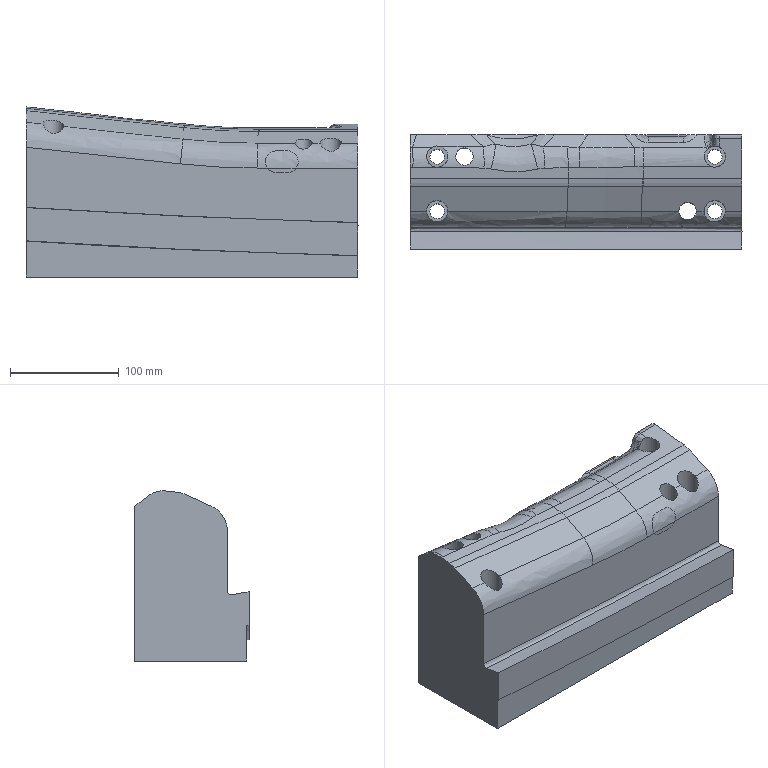Part | NX | features solid 2 | 1 solid | 80 faces | box 305 x 104.845 x 156.412 mm | volume 3602873 mm3 | spline 62 | cylinder 10 | plane 8 | commonest cylinder face diameters 13.5 x4 19.5 x4 16 x2